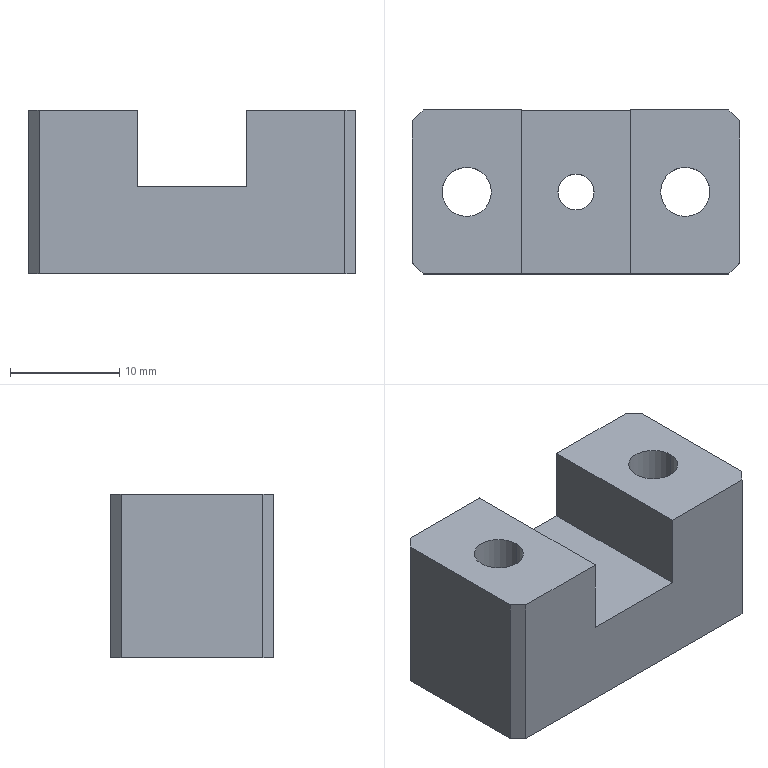Part | STEP file | 03-11 upper blade limit block | 1 solid | 26 faces | box 30 x 15 x 15 mm | volume 4822 mm3 | plane 16 | cylinder 10 | commonest cylinder face diameters 4.5 x4 8 x4 3.3 x2
STEP:
#1=CARTESIAN_POINT('',(-6.,0.,4.4));
#2=VERTEX_POINT('',#1);
#3=CARTESIAN_POINT('',(-14.,0.,4.4));
#4=VERTEX_POINT('',#3);
#5=CARTESIAN_POINT('',(-10.,0.,4.4));
#6=DIRECTION('',(0.,0.,-1.));
#7=DIRECTION('',(-1.,0.,0.));
#8=AXIS2_PLACEMENT_3D('',#5,#6,#7);
#9=CIRCLE('',#8,4.);
#10=EDGE_CURVE('',#2,#4,#9,.T.);
#11=ORIENTED_EDGE('',*,*,#10,.F.);
#12=CARTESIAN_POINT('',(-6.,0.,0.));
#13=VERTEX_POINT('',#12);
#14=CARTESIAN_POINT('',(-6.,0.,0.));
#15=DIRECTION('',(0.,0.,-1.));
#16=VECTOR('',#15,1000.);
#17=LINE('',#14,#16);
#18=EDGE_CURVE('',#2,#13,#17,.T.);
#19=ORIENTED_EDGE('',*,*,#18,.T.);
#20=CARTESIAN_POINT('',(-14.,0.,0.));
#21=VERTEX_POINT('',#20);
#22=CARTESIAN_POINT('',(-10.,0.,0.));
#23=DIRECTION('',(0.,0.,-1.));
#24=DIRECTION('',(-1.,0.,0.));
#25=AXIS2_PLACEMENT_3D('',#22,#23,#24);
#26=CIRCLE('',#25,4.);
#27=EDGE_CURVE('',#13,#21,#26,.T.);
#28=ORIENTED_EDGE('',*,*,#27,.T.);
#29=CARTESIAN_POINT('',(-14.,0.,0.));
#30=DIRECTION('',(0.,0.,-1.));
#31=VECTOR('',#30,1000.);
#32=LINE('',#29,#31);
#33=EDGE_CURVE('',#4,#21,#32,.T.);
#34=ORIENTED_EDGE('',*,*,#33,.F.);
#35=EDGE_LOOP('',(#11,#19,#28,#34));
#36=FACE_OUTER_BOUND('',#35,.T.);
#37=CARTESIAN_POINT('',(-10.,0.,0.));
#38=DIRECTION('',(0.,0.,-1.));
#39=DIRECTION('',(-1.,0.,0.));
#40=AXIS2_PLACEMENT_3D('',#37,#38,#39);
#41=CYLINDRICAL_SURFACE('',#40,4.);
#42=ADVANCED_FACE('',(#36),#41,.F.);
#43=CARTESIAN_POINT('',(-7.75,0.,15.));
#44=VERTEX_POINT('',#43);
#45=CARTESIAN_POINT('',(-12.25,0.,15.));
#46=VERTEX_POINT('',#45);
#47=CARTESIAN_POINT('',(-10.,0.,15.));
#48=DIRECTION('',(0.,0.,-1.));
#49=DIRECTION('',(-1.,0.,0.));
#50=AXIS2_PLACEMENT_3D('',#47,#48,#49);
#51=CIRCLE('',#50,2.25);
#52=EDGE_CURVE('',#44,#46,#51,.T.);
#53=ORIENTED_EDGE('',*,*,#52,.F.);
#54=CARTESIAN_POINT('',(-7.75,0.,4.4));
#55=VERTEX_POINT('',#54);
#56=CARTESIAN_POINT('',(-7.75,0.,0.));
#57=DIRECTION('',(0.,0.,-1.));
#58=VECTOR('',#57,1000.);
#59=LINE('',#56,#58);
#60=EDGE_CURVE('',#44,#55,#59,.T.);
#61=ORIENTED_EDGE('',*,*,#60,.T.);
#62=CARTESIAN_POINT('',(-12.25,0.,4.4));
#63=VERTEX_POINT('',#62);
#64=CARTESIAN_POINT('',(-10.,0.,4.4));
#65=DIRECTION('',(0.,0.,-1.));
#66=DIRECTION('',(-1.,0.,0.));
#67=AXIS2_PLACEMENT_3D('',#64,#65,#66);
#68=CIRCLE('',#67,2.25);
#69=EDGE_CURVE('',#55,#63,#68,.T.);
#70=ORIENTED_EDGE('',*,*,#69,.T.);
#71=CARTESIAN_POINT('',(-12.25,0.,0.));
#72=DIRECTION('',(0.,0.,-1.));
#73=VECTOR('',#72,1000.);
#74=LINE('',#71,#73);
#75=EDGE_CURVE('',#46,#63,#74,.T.);
#76=ORIENTED_EDGE('',*,*,#75,.F.);
#77=EDGE_LOOP('',(#53,#61,#70,#76));
#78=FACE_OUTER_BOUND('',#77,.T.);
#79=CARTESIAN_POINT('',(-10.,0.,0.));
#80=DIRECTION('',(0.,0.,-1.));
#81=DIRECTION('',(-1.,0.,0.));
#82=AXIS2_PLACEMENT_3D('',#79,#80,#81);
#83=CYLINDRICAL_SURFACE('',#82,2.25);
#84=ADVANCED_FACE('',(#78),#83,.F.);
#85=CARTESIAN_POINT('',(14.,0.,4.4));
#86=VERTEX_POINT('',#85);
#87=CARTESIAN_POINT('',(6.,0.,4.4));
#88=VERTEX_POINT('',#87);
#89=CARTESIAN_POINT('',(10.,0.,4.4));
#90=DIRECTION('',(0.,0.,-1.));
#91=DIRECTION('',(-1.,0.,0.));
#92=AXIS2_PLACEMENT_3D('',#89,#90,#91);
#93=CIRCLE('',#92,4.);
#94=EDGE_CURVE('',#86,#88,#93,.T.);
#95=ORIENTED_EDGE('',*,*,#94,.F.);
#96=CARTESIAN_POINT('',(14.,0.,0.));
#97=VERTEX_POINT('',#96);
#98=CARTESIAN_POINT('',(14.,0.,0.));
#99=DIRECTION('',(0.,0.,-1.));
#100=VECTOR('',#99,1000.);
#101=LINE('',#98,#100);
#102=EDGE_CURVE('',#86,#97,#101,.T.);
#103=ORIENTED_EDGE('',*,*,#102,.T.);
#104=CARTESIAN_POINT('',(6.,0.,0.));
#105=VERTEX_POINT('',#104);
#106=CARTESIAN_POINT('',(10.,0.,0.));
#107=DIRECTION('',(0.,0.,-1.));
#108=DIRECTION('',(-1.,0.,0.));
#109=AXIS2_PLACEMENT_3D('',#106,#107,#108);
#110=CIRCLE('',#109,4.);
#111=EDGE_CURVE('',#97,#105,#110,.T.);
#112=ORIENTED_EDGE('',*,*,#111,.T.);
#113=CARTESIAN_POINT('',(6.,0.,0.));
#114=DIRECTION('',(0.,0.,-1.));
#115=VECTOR('',#114,1000.);
#116=LINE('',#113,#115);
#117=EDGE_CURVE('',#88,#105,#116,.T.);
#118=ORIENTED_EDGE('',*,*,#117,.F.);
#119=EDGE_LOOP('',(#95,#103,#112,#118));
#120=FACE_OUTER_BOUND('',#119,.T.);
#121=CARTESIAN_POINT('',(10.,0.,0.));
#122=DIRECTION('',(0.,0.,-1.));
#123=DIRECTION('',(-1.,0.,0.));
#124=AXIS2_PLACEMENT_3D('',#121,#122,#123);
#125=CYLINDRICAL_SURFACE('',#124,4.);
#126=ADVANCED_FACE('',(#120),#125,.F.);
#127=CARTESIAN_POINT('',(12.25,0.,15.));
#128=VERTEX_POINT('',#127);
#129=CARTESIAN_POINT('',(7.75,0.,15.));
#130=VERTEX_POINT('',#129);
#131=CARTESIAN_POINT('',(10.,0.,15.));
#132=DIRECTION('',(0.,0.,-1.));
#133=DIRECTION('',(-1.,0.,0.));
#134=AXIS2_PLACEMENT_3D('',#131,#132,#133);
#135=CIRCLE('',#134,2.25);
#136=EDGE_CURVE('',#128,#130,#135,.T.);
#137=ORIENTED_EDGE('',*,*,#136,.F.);
#138=CARTESIAN_POINT('',(12.25,0.,4.4));
#139=VERTEX_POINT('',#138);
#140=CARTESIAN_POINT('',(12.25,0.,0.));
#141=DIRECTION('',(0.,0.,-1.));
#142=VECTOR('',#141,1000.);
#143=LINE('',#140,#142);
#144=EDGE_CURVE('',#128,#139,#143,.T.);
#145=ORIENTED_EDGE('',*,*,#144,.T.);
#146=CARTESIAN_POINT('',(7.75,0.,4.4));
#147=VERTEX_POINT('',#146);
#148=CARTESIAN_POINT('',(10.,0.,4.4));
#149=DIRECTION('',(0.,0.,-1.));
#150=DIRECTION('',(-1.,0.,0.));
#151=AXIS2_PLACEMENT_3D('',#148,#149,#150);
#152=CIRCLE('',#151,2.25);
#153=EDGE_CURVE('',#139,#147,#152,.T.);
#154=ORIENTED_EDGE('',*,*,#153,.T.);
#155=CARTESIAN_POINT('',(7.75,0.,0.));
#156=DIRECTION('',(0.,0.,-1.));
#157=VECTOR('',#156,1000.);
#158=LINE('',#155,#157);
#159=EDGE_CURVE('',#130,#147,#158,.T.);
#160=ORIENTED_EDGE('',*,*,#159,.F.);
#161=EDGE_LOOP('',(#137,#145,#154,#160));
#162=FACE_OUTER_BOUND('',#161,.T.);
#163=CARTESIAN_POINT('',(10.,0.,0.));
#164=DIRECTION('',(0.,0.,-1.));
#165=DIRECTION('',(-1.,0.,0.));
#166=AXIS2_PLACEMENT_3D('',#163,#164,#165);
#167=CYLINDRICAL_SURFACE('',#166,2.25);
#168=ADVANCED_FACE('',(#162),#167,.F.);
#169=CARTESIAN_POINT('',(1.65,0.,8.));
#170=VERTEX_POINT('',#169);
#171=CARTESIAN_POINT('',(-1.65,0.,8.));
#172=VERTEX_POINT('',#171);
#173=CARTESIAN_POINT('',(0.,0.,8.));
#174=DIRECTION('',(0.,0.,-1.));
#175=DIRECTION('',(-1.,0.,0.));
#176=AXIS2_PLACEMENT_3D('',#173,#174,#175);
#177=CIRCLE('',#176,1.65);
#178=EDGE_CURVE('',#170,#172,#177,.T.);
#179=ORIENTED_EDGE('',*,*,#178,.F.);
#180=CARTESIAN_POINT('',(1.65,0.,0.));
#181=VERTEX_POINT('',#180);
#182=CARTESIAN_POINT('',(1.65,0.,0.));
#183=DIRECTION('',(0.,0.,-1.));
#184=VECTOR('',#183,1000.);
#185=LINE('',#182,#184);
#186=EDGE_CURVE('',#170,#181,#185,.T.);
#187=ORIENTED_EDGE('',*,*,#186,.T.);
#188=CARTESIAN_POINT('',(-1.65,0.,0.));
#189=VERTEX_POINT('',#188);
#190=CARTESIAN_POINT('',(0.,0.,0.));
#191=DIRECTION('',(0.,0.,-1.));
#192=DIRECTION('',(-1.,0.,0.));
#193=AXIS2_PLACEMENT_3D('',#190,#191,#192);
#194=CIRCLE('',#193,1.65);
#195=EDGE_CURVE('',#181,#189,#194,.T.);
#196=ORIENTED_EDGE('',*,*,#195,.T.);
#197=CARTESIAN_POINT('',(-1.65,0.,0.));
#198=DIRECTION('',(0.,0.,-1.));
#199=VECTOR('',#198,1000.);
#200=LINE('',#197,#199);
#201=EDGE_CURVE('',#172,#189,#200,.T.);
#202=ORIENTED_EDGE('',*,*,#201,.F.);
#203=EDGE_LOOP('',(#179,#187,#196,#202));
#204=FACE_OUTER_BOUND('',#203,.T.);
#205=CARTESIAN_POINT('',(0.,0.,0.));
#206=DIRECTION('',(0.,0.,-1.));
#207=DIRECTION('',(-1.,0.,0.));
#208=AXIS2_PLACEMENT_3D('',#205,#206,#207);
#209=CYLINDRICAL_SURFACE('',#208,1.65);
#210=ADVANCED_FACE('',(#204),#209,.F.);
#211=CARTESIAN_POINT('',(-10.,0.,15.));
#212=DIRECTION('',(0.,0.,-1.));
#213=DIRECTION('',(-1.,0.,0.));
#214=AXIS2_PLACEMENT_3D('',#211,#212,#213);
#215=CIRCLE('',#214,2.25);
#216=EDGE_CURVE('',#46,#44,#215,.T.);
#217=ORIENTED_EDGE('',*,*,#216,.T.);
#218=ORIENTED_EDGE('',*,*,#52,.T.);
#219=EDGE_LOOP('',(#217,#218));
#220=FACE_BOUND('',#219,.T.);
#221=CARTESIAN_POINT('',(-15.,6.5,15.));
#222=VERTEX_POINT('',#221);
#223=CARTESIAN_POINT('',(-15.,-6.5,15.));
#224=VERTEX_POINT('',#223);
#225=CARTESIAN_POINT('',(-15.,7.5,15.));
#226=DIRECTION('',(0.,-1.,0.));
#227=VECTOR('',#226,1000.);
#228=LINE('',#225,#227);
#229=EDGE_CURVE('',#222,#224,#228,.T.);
#230=ORIENTED_EDGE('',*,*,#229,.T.);
#231=CARTESIAN_POINT('',(-14.,-7.5,15.));
#232=VERTEX_POINT('',#231);
#233=CARTESIAN_POINT('',(0.5,-22.,15.));
#234=DIRECTION('',(0.7071,-0.7071,0.));
#235=VECTOR('',#234,1000.);
#236=LINE('',#233,#235);
#237=EDGE_CURVE('',#224,#232,#236,.T.);
#238=ORIENTED_EDGE('',*,*,#237,.T.);
#239=CARTESIAN_POINT('',(-5.,-7.5,15.));
#240=VERTEX_POINT('',#239);
#241=CARTESIAN_POINT('',(-15.,-7.5,15.));
#242=DIRECTION('',(1.,0.,0.));
#243=VECTOR('',#242,1000.);
#244=LINE('',#241,#243);
#245=EDGE_CURVE('',#232,#240,#244,.T.);
#246=ORIENTED_EDGE('',*,*,#245,.T.);
#247=CARTESIAN_POINT('',(-5.,7.5,15.));
#248=VERTEX_POINT('',#247);
#249=CARTESIAN_POINT('',(-5.,7.5,15.));
#250=DIRECTION('',(0.,-1.,0.));
#251=VECTOR('',#250,1000.);
#252=LINE('',#249,#251);
#253=EDGE_CURVE('',#248,#240,#252,.T.);
#254=ORIENTED_EDGE('',*,*,#253,.F.);
#255=CARTESIAN_POINT('',(-14.,7.5,15.));
#256=VERTEX_POINT('',#255);
#257=CARTESIAN_POINT('',(-15.,7.5,15.));
#258=DIRECTION('',(-1.,0.,0.));
#259=VECTOR('',#258,1000.);
#260=LINE('',#257,#259);
#261=EDGE_CURVE('',#248,#256,#260,.T.);
#262=ORIENTED_EDGE('',*,*,#261,.T.);
#263=CARTESIAN_POINT('',(-7.,14.5,15.));
#264=DIRECTION('',(-0.7071,-0.7071,0.));
#265=VECTOR('',#264,1000.);
#266=LINE('',#263,#265);
#267=EDGE_CURVE('',#256,#222,#266,.T.);
#268=ORIENTED_EDGE('',*,*,#267,.T.);
#269=EDGE_LOOP('',(#230,#238,#246,#254,#262,#268));
#270=FACE_OUTER_BOUND('',#269,.T.);
#271=CARTESIAN_POINT('',(15.,-7.5,15.));
#272=DIRECTION('',(0.,0.,1.));
#273=DIRECTION('',(1.,0.,0.));
#274=AXIS2_PLACEMENT_3D('',#271,#272,#273);
#275=PLANE('',#274);
#276=ADVANCED_FACE('',(#220,#270),#275,.T.);
#277=CARTESIAN_POINT('',(15.,-6.5,15.));
#278=VERTEX_POINT('',#277);
#279=CARTESIAN_POINT('',(15.,6.5,15.));
#280=VERTEX_POINT('',#279);
#281=CARTESIAN_POINT('',(15.,7.5,15.));
#282=DIRECTION('',(0.,1.,0.));
#283=VECTOR('',#282,1000.);
#284=LINE('',#281,#283);
#285=EDGE_CURVE('',#278,#280,#284,.T.);
#286=ORIENTED_EDGE('',*,*,#285,.F.);
#287=CARTESIAN_POINT('',(15.,-6.5,0.));
#288=VERTEX_POINT('',#287);
#289=CARTESIAN_POINT('',(15.,-6.5,15.));
#290=DIRECTION('',(0.,0.,-1.));
#291=VECTOR('',#290,1000.);
#292=LINE('',#289,#291);
#293=EDGE_CURVE('',#278,#288,#292,.T.);
#294=ORIENTED_EDGE('',*,*,#293,.T.);
#295=CARTESIAN_POINT('',(15.,6.5,0.));
#296=VERTEX_POINT('',#295);
#297=CARTESIAN_POINT('',(15.,7.5,0.));
#298=DIRECTION('',(0.,1.,0.));
#299=VECTOR('',#298,1000.);
#300=LINE('',#297,#299);
#301=EDGE_CURVE('',#288,#296,#300,.T.);
#302=ORIENTED_EDGE('',*,*,#301,.T.);
#303=CARTESIAN_POINT('',(15.,6.5,15.));
#304=DIRECTION('',(0.,0.,1.));
#305=VECTOR('',#304,1000.);
#306=LINE('',#303,#305);
#307=EDGE_CURVE('',#296,#280,#306,.T.);
#308=ORIENTED_EDGE('',*,*,#307,.T.);
#309=EDGE_LOOP('',(#286,#294,#302,#308));
#310=FACE_OUTER_BOUND('',#309,.T.);
#311=CARTESIAN_POINT('',(15.,7.5,15.));
#312=DIRECTION('',(-1.,0.,0.));
#313=DIRECTION('',(0.,-1.,0.));
#314=AXIS2_PLACEMENT_3D('',#311,#312,#313);
#315=PLANE('',#314);
#316=ADVANCED_FACE('',(#310),#315,.F.);
#317=CARTESIAN_POINT('',(14.,7.5,15.));
#318=VERTEX_POINT('',#317);
#319=CARTESIAN_POINT('',(5.,7.5,15.));
#320=VERTEX_POINT('',#319);
#321=CARTESIAN_POINT('',(-15.,7.5,15.));
#322=DIRECTION('',(-1.,0.,0.));
#323=VECTOR('',#322,1000.);
#324=LINE('',#321,#323);
#325=EDGE_CURVE('',#318,#320,#324,.T.);
#326=ORIENTED_EDGE('',*,*,#325,.F.);
#327=CARTESIAN_POINT('',(14.,7.5,0.));
#328=VERTEX_POINT('',#327);
#329=CARTESIAN_POINT('',(14.,7.5,15.));
#330=DIRECTION('',(0.,0.,-1.));
#331=VECTOR('',#330,1000.);
#332=LINE('',#329,#331);
#333=EDGE_CURVE('',#318,#328,#332,.T.);
#334=ORIENTED_EDGE('',*,*,#333,.T.);
#335=CARTESIAN_POINT('',(-14.,7.5,0.));
#336=VERTEX_POINT('',#335);
#337=CARTESIAN_POINT('',(-15.,7.5,0.));
#338=DIRECTION('',(-1.,0.,0.));
#339=VECTOR('',#338,1000.);
#340=LINE('',#337,#339);
#341=EDGE_CURVE('',#328,#336,#340,.T.);
#342=ORIENTED_EDGE('',*,*,#341,.T.);
#343=CARTESIAN_POINT('',(-14.,7.5,15.));
#344=DIRECTION('',(0.,0.,1.));
#345=VECTOR('',#344,1000.);
#346=LINE('',#343,#345);
#347=EDGE_CURVE('',#336,#256,#346,.T.);
#348=ORIENTED_EDGE('',*,*,#347,.T.);
#349=ORIENTED_EDGE('',*,*,#261,.F.);
#350=CARTESIAN_POINT('',(-5.,7.5,8.));
#351=VERTEX_POINT('',#350);
#352=CARTESIAN_POINT('',(-5.,7.5,15.));
#353=DIRECTION('',(0.,0.,-1.));
#354=VECTOR('',#353,1000.);
#355=LINE('',#352,#354);
#356=EDGE_CURVE('',#248,#351,#355,.T.);
#357=ORIENTED_EDGE('',*,*,#356,.T.);
#358=CARTESIAN_POINT('',(5.,7.5,8.));
#359=VERTEX_POINT('',#358);
#360=CARTESIAN_POINT('',(-5.,7.5,8.));
#361=DIRECTION('',(1.,0.,0.));
#362=VECTOR('',#361,1000.);
#363=LINE('',#360,#362);
#364=EDGE_CURVE('',#351,#359,#363,.T.);
#365=ORIENTED_EDGE('',*,*,#364,.T.);
#366=CARTESIAN_POINT('',(5.,7.5,15.));
#367=DIRECTION('',(0.,0.,1.));
#368=VECTOR('',#367,1000.);
#369=LINE('',#366,#368);
#370=EDGE_CURVE('',#359,#320,#369,.T.);
#371=ORIENTED_EDGE('',*,*,#370,.T.);
#372=EDGE_LOOP('',(#326,#334,#342,#348,#349,#357,#365,#371));
#373=FACE_OUTER_BOUND('',#372,.T.);
#374=CARTESIAN_POINT('',(-15.,7.5,15.));
#375=DIRECTION('',(0.,-1.,0.));
#376=DIRECTION('',(0.,0.,-1.));
#377=AXIS2_PLACEMENT_3D('',#374,#375,#376);
#378=PLANE('',#377);
#379=ADVANCED_FACE('',(#373),#378,.F.);
#380=CARTESIAN_POINT('',(-15.,6.5,0.));
#381=VERTEX_POINT('',#380);
#382=CARTESIAN_POINT('',(-15.,-6.5,0.));
#383=VERTEX_POINT('',#382);
#384=CARTESIAN_POINT('',(-15.,7.5,0.));
#385=DIRECTION('',(0.,-1.,0.));
#386=VECTOR('',#385,1000.);
#387=LINE('',#384,#386);
#388=EDGE_CURVE('',#381,#383,#387,.T.);
#389=ORIENTED_EDGE('',*,*,#388,.T.);
#390=CARTESIAN_POINT('',(-15.,-6.5,15.));
#391=DIRECTION('',(0.,0.,1.));
#392=VECTOR('',#391,1000.);
#393=LINE('',#390,#392);
#394=EDGE_CURVE('',#383,#224,#393,.T.);
#395=ORIENTED_EDGE('',*,*,#394,.T.);
#396=ORIENTED_EDGE('',*,*,#229,.F.);
#397=CARTESIAN_POINT('',(-15.,6.5,15.));
#398=DIRECTION('',(0.,0.,-1.));
#399=VECTOR('',#398,1000.);
#400=LINE('',#397,#399);
#401=EDGE_CURVE('',#222,#381,#400,.T.);
#402=ORIENTED_EDGE('',*,*,#401,.T.);
#403=EDGE_LOOP('',(#389,#395,#396,#402));
#404=FACE_OUTER_BOUND('',#403,.T.);
#405=CARTESIAN_POINT('',(-15.,7.5,15.));
#406=DIRECTION('',(1.,0.,0.));
#407=DIRECTION('',(0.,1.,0.));
#408=AXIS2_PLACEMENT_3D('',#405,#406,#407);
#409=PLANE('',#408);
#410=ADVANCED_FACE('',(#404),#409,.F.);
#411=ORIENTED_EDGE('',*,*,#245,.F.);
#412=CARTESIAN_POINT('',(-14.,-7.5,0.));
#413=VERTEX_POINT('',#412);
#414=CARTESIAN_POINT('',(-14.,-7.5,15.));
#415=DIRECTION('',(0.,0.,-1.));
#416=VECTOR('',#415,1000.);
#417=LINE('',#414,#416);
#418=EDGE_CURVE('',#232,#413,#417,.T.);
#419=ORIENTED_EDGE('',*,*,#418,.T.);
#420=CARTESIAN_POINT('',(14.,-7.5,0.));
#421=VERTEX_POINT('',#420);
#422=CARTESIAN_POINT('',(-15.,-7.5,0.));
#423=DIRECTION('',(1.,0.,0.));
#424=VECTOR('',#423,1000.);
#425=LINE('',#422,#424);
#426=EDGE_CURVE('',#413,#421,#425,.T.);
#427=ORIENTED_EDGE('',*,*,#426,.T.);
#428=CARTESIAN_POINT('',(14.,-7.5,15.));
#429=VERTEX_POINT('',#428);
#430=CARTESIAN_POINT('',(14.,-7.5,15.));
#431=DIRECTION('',(0.,0.,1.));
#432=VECTOR('',#431,1000.);
#433=LINE('',#430,#432);
#434=EDGE_CURVE('',#421,#429,#433,.T.);
#435=ORIENTED_EDGE('',*,*,#434,.T.);
#436=CARTESIAN_POINT('',(5.,-7.5,15.));
#437=VERTEX_POINT('',#436);
#438=CARTESIAN_POINT('',(-15.,-7.5,15.));
#439=DIRECTION('',(1.,0.,0.));
#440=VECTOR('',#439,1000.);
#441=LINE('',#438,#440);
#442=EDGE_CURVE('',#437,#429,#441,.T.);
#443=ORIENTED_EDGE('',*,*,#442,.F.);
#444=CARTESIAN_POINT('',(5.,-7.5,8.));
#445=VERTEX_POINT('',#444);
#446=CARTESIAN_POINT('',(5.,-7.5,15.));
#447=DIRECTION('',(0.,0.,1.));
#448=VECTOR('',#447,1000.);
#449=LINE('',#446,#448);
#450=EDGE_CURVE('',#445,#437,#449,.T.);
#451=ORIENTED_EDGE('',*,*,#450,.F.);
#452=CARTESIAN_POINT('',(-5.,-7.5,8.));
#453=VERTEX_POINT('',#452);
#454=CARTESIAN_POINT('',(-5.,-7.5,8.));
#455=DIRECTION('',(1.,0.,0.));
#456=VECTOR('',#455,1000.);
#457=LINE('',#454,#456);
#458=EDGE_CURVE('',#453,#445,#457,.T.);
#459=ORIENTED_EDGE('',*,*,#458,.F.);
#460=CARTESIAN_POINT('',(-5.,-7.5,15.));
#461=DIRECTION('',(0.,0.,-1.));
#462=VECTOR('',#461,1000.);
#463=LINE('',#460,#462);
#464=EDGE_CURVE('',#240,#453,#463,.T.);
#465=ORIENTED_EDGE('',*,*,#464,.F.);
#466=EDGE_LOOP('',(#411,#419,#427,#435,#443,#451,#459,#465));
#467=FACE_OUTER_BOUND('',#466,.T.);
#468=CARTESIAN_POINT('',(-15.,-7.5,15.));
#469=DIRECTION('',(0.,1.,0.));
#470=DIRECTION('',(0.,0.,1.));
#471=AXIS2_PLACEMENT_3D('',#468,#469,#470);
#472=PLANE('',#471);
#473=ADVANCED_FACE('',(#467),#472,.F.);
#474=CARTESIAN_POINT('',(10.,0.,15.));
#475=DIRECTION('',(0.,0.,-1.));
#476=DIRECTION('',(-1.,0.,0.));
#477=AXIS2_PLACEMENT_3D('',#474,#475,#476);
#478=CIRCLE('',#477,2.25);
#479=EDGE_CURVE('',#130,#128,#478,.T.);
#480=ORIENTED_EDGE('',*,*,#479,.T.);
#481=ORIENTED_EDGE('',*,*,#136,.T.);
#482=EDGE_LOOP('',(#480,#481));
#483=FACE_BOUND('',#482,.T.);
#484=ORIENTED_EDGE('',*,*,#442,.T.);
#485=CARTESIAN_POINT('',(14.5,-7.,15.));
#486=DIRECTION('',(0.7071,0.7071,0.));
#487=VECTOR('',#486,1000.);
#488=LINE('',#485,#487);
#489=EDGE_CURVE('',#429,#278,#488,.T.);
#490=ORIENTED_EDGE('',*,*,#489,.T.);
#491=ORIENTED_EDGE('',*,*,#285,.T.);
#492=CARTESIAN_POINT('',(22.,-0.5,15.));
#493=DIRECTION('',(-0.7071,0.7071,0.));
#494=VECTOR('',#493,1000.);
#495=LINE('',#492,#494);
#496=EDGE_CURVE('',#280,#318,#495,.T.);
#497=ORIENTED_EDGE('',*,*,#496,.T.);
#498=ORIENTED_EDGE('',*,*,#325,.T.);
#499=CARTESIAN_POINT('',(5.,7.5,15.));
#500=DIRECTION('',(0.,-1.,0.));
#501=VECTOR('',#500,1000.);
#502=LINE('',#499,#501);
#503=EDGE_CURVE('',#320,#437,#502,.T.);
#504=ORIENTED_EDGE('',*,*,#503,.T.);
#505=EDGE_LOOP('',(#484,#490,#491,#497,#498,#504));
#506=FACE_OUTER_BOUND('',#505,.T.);
#507=CARTESIAN_POINT('',(15.,-7.5,15.));
#508=DIRECTION('',(0.,0.,1.));
#509=DIRECTION('',(1.,0.,0.));
#510=AXIS2_PLACEMENT_3D('',#507,#508,#509);
#511=PLANE('',#510);
#512=ADVANCED_FACE('',(#483,#506),#511,.T.);
#513=CARTESIAN_POINT('',(-10.,0.,0.));
#514=DIRECTION('',(0.,0.,-1.));
#515=DIRECTION('',(-1.,0.,0.));
#516=AXIS2_PLACEMENT_3D('',#513,#514,#515);
#517=CIRCLE('',#516,4.);
#518=EDGE_CURVE('',#21,#13,#517,.T.);
#519=ORIENTED_EDGE('',*,*,#518,.F.);
#520=ORIENTED_EDGE('',*,*,#27,.F.);
#521=EDGE_LOOP('',(#519,#520));
#522=FACE_BOUND('',#521,.T.);
#523=CARTESIAN_POINT('',(10.,0.,0.));
#524=DIRECTION('',(0.,0.,-1.));
#525=DIRECTION('',(-1.,0.,0.));
#526=AXIS2_PLACEMENT_3D('',#523,#524,#525);
#527=CIRCLE('',#526,4.);
#528=EDGE_CURVE('',#105,#97,#527,.T.);
#529=ORIENTED_EDGE('',*,*,#528,.F.);
#530=ORIENTED_EDGE('',*,*,#111,.F.);
#531=EDGE_LOOP('',(#529,#530));
#532=FACE_BOUND('',#531,.T.);
#533=CARTESIAN_POINT('',(0.,0.,0.));
#534=DIRECTION('',(0.,0.,-1.));
#535=DIRECTION('',(-1.,0.,0.));
#536=AXIS2_PLACEMENT_3D('',#533,#534,#535);
#537=CIRCLE('',#536,1.65);
#538=EDGE_CURVE('',#189,#181,#537,.T.);
#539=ORIENTED_EDGE('',*,*,#538,.F.);
#540=ORIENTED_EDGE('',*,*,#195,.F.);
#541=EDGE_LOOP('',(#539,#540));
#542=FACE_BOUND('',#541,.T.);
#543=ORIENTED_EDGE('',*,*,#426,.F.);
#544=CARTESIAN_POINT('',(-14.,-7.5,0.));
#545=DIRECTION('',(-0.7071,0.7071,0.));
#546=VECTOR('',#545,1000.);
#547=LINE('',#544,#546);
#548=EDGE_CURVE('',#413,#383,#547,.T.);
#549=ORIENTED_EDGE('',*,*,#548,.T.);
#550=ORIENTED_EDGE('',*,*,#388,.F.);
#551=CARTESIAN_POINT('',(-15.,6.5,0.));
#552=DIRECTION('',(0.7071,0.7071,0.));
#553=VECTOR('',#552,1000.);
#554=LINE('',#551,#553);
#555=EDGE_CURVE('',#381,#336,#554,.T.);
#556=ORIENTED_EDGE('',*,*,#555,.T.);
#557=ORIENTED_EDGE('',*,*,#341,.F.);
#558=CARTESIAN_POINT('',(14.,7.5,0.));
#559=DIRECTION('',(0.7071,-0.7071,0.));
#560=VECTOR('',#559,1000.);
#561=LINE('',#558,#560);
#562=EDGE_CURVE('',#328,#296,#561,.T.);
#563=ORIENTED_EDGE('',*,*,#562,.T.);
#564=ORIENTED_EDGE('',*,*,#301,.F.);
#565=CARTESIAN_POINT('',(15.,-6.5,0.));
#566=DIRECTION('',(-0.7071,-0.7071,0.));
#567=VECTOR('',#566,1000.);
#568=LINE('',#565,#567);
#569=EDGE_CURVE('',#288,#421,#568,.T.);
#570=ORIENTED_EDGE('',*,*,#569,.T.);
#571=EDGE_LOOP('',(#543,#549,#550,#556,#557,#563,#564,#570));
#572=FACE_OUTER_BOUND('',#571,.T.);
#573=CARTESIAN_POINT('',(15.,-7.5,0.));
#574=DIRECTION('',(0.,0.,1.));
#575=DIRECTION('',(1.,0.,0.));
#576=AXIS2_PLACEMENT_3D('',#573,#574,#575);
#577=PLANE('',#576);
#578=ADVANCED_FACE('',(#522,#532,#542,#572),#577,.F.);
#579=ORIENTED_EDGE('',*,*,#464,.T.);
#580=CARTESIAN_POINT('',(-5.,7.5,8.));
#581=DIRECTION('',(0.,-1.,0.));
#582=VECTOR('',#581,1000.);
#583=LINE('',#580,#582);
#584=EDGE_CURVE('',#351,#453,#583,.T.);
#585=ORIENTED_EDGE('',*,*,#584,.F.);
#586=ORIENTED_EDGE('',*,*,#356,.F.);
#587=ORIENTED_EDGE('',*,*,#253,.T.);
#588=EDGE_LOOP('',(#579,#585,#586,#587));
#589=FACE_OUTER_BOUND('',#588,.T.);
#590=CARTESIAN_POINT('',(-5.,7.5,15.));
#591=DIRECTION('',(-1.,0.,0.));
#592=DIRECTION('',(0.,0.,1.));
#593=AXIS2_PLACEMENT_3D('',#590,#591,#592);
#594=PLANE('',#593);
#595=ADVANCED_FACE('',(#589),#594,.F.);
#596=ORIENTED_EDGE('',*,*,#450,.T.);
#597=ORIENTED_EDGE('',*,*,#503,.F.);
#598=ORIENTED_EDGE('',*,*,#370,.F.);
#599=CARTESIAN_POINT('',(5.,7.5,8.));
#600=DIRECTION('',(0.,-1.,0.));
#601=VECTOR('',#600,1000.);
#602=LINE('',#599,#601);
#603=EDGE_CURVE('',#359,#445,#602,.T.);
#604=ORIENTED_EDGE('',*,*,#603,.T.);
#605=EDGE_LOOP('',(#596,#597,#598,#604));
#606=FACE_OUTER_BOUND('',#605,.T.);
#607=CARTESIAN_POINT('',(5.,7.5,15.));
#608=DIRECTION('',(1.,0.,0.));
#609=DIRECTION('',(0.,0.,-1.));
#610=AXIS2_PLACEMENT_3D('',#607,#608,#609);
#611=PLANE('',#610);
#612=ADVANCED_FACE('',(#606),#611,.F.);
#613=CARTESIAN_POINT('',(0.,0.,8.));
#614=DIRECTION('',(0.,0.,-1.));
#615=DIRECTION('',(-1.,0.,0.));
#616=AXIS2_PLACEMENT_3D('',#613,#614,#615);
#617=CIRCLE('',#616,1.65);
#618=EDGE_CURVE('',#172,#170,#617,.T.);
#619=ORIENTED_EDGE('',*,*,#618,.T.);
#620=ORIENTED_EDGE('',*,*,#178,.T.);
#621=EDGE_LOOP('',(#619,#620));
#622=FACE_BOUND('',#621,.T.);
#623=ORIENTED_EDGE('',*,*,#458,.T.);
#624=ORIENTED_EDGE('',*,*,#603,.F.);
#625=ORIENTED_EDGE('',*,*,#364,.F.);
#626=ORIENTED_EDGE('',*,*,#584,.T.);
#627=EDGE_LOOP('',(#623,#624,#625,#626));
#628=FACE_OUTER_BOUND('',#627,.T.);
#629=CARTESIAN_POINT('',(-5.,7.5,8.));
#630=DIRECTION('',(0.,0.,-1.));
#631=DIRECTION('',(-1.,0.,0.));
#632=AXIS2_PLACEMENT_3D('',#629,#630,#631);
#633=PLANE('',#632);
#634=ADVANCED_FACE('',(#622,#628),#633,.F.);
#635=ORIENTED_EDGE('',*,*,#186,.F.);
#636=ORIENTED_EDGE('',*,*,#618,.F.);
#637=ORIENTED_EDGE('',*,*,#201,.T.);
#638=ORIENTED_EDGE('',*,*,#538,.T.);
#639=EDGE_LOOP('',(#635,#636,#637,#638));
#640=FACE_OUTER_BOUND('',#639,.T.);
#641=CARTESIAN_POINT('',(0.,0.,0.));
#642=DIRECTION('',(0.,0.,-1.));
#643=DIRECTION('',(-1.,0.,0.));
#644=AXIS2_PLACEMENT_3D('',#641,#642,#643);
#645=CYLINDRICAL_SURFACE('',#644,1.65);
#646=ADVANCED_FACE('',(#640),#645,.F.);
#647=ORIENTED_EDGE('',*,*,#237,.F.);
#648=ORIENTED_EDGE('',*,*,#394,.F.);
#649=ORIENTED_EDGE('',*,*,#548,.F.);
#650=ORIENTED_EDGE('',*,*,#418,.F.);
#651=EDGE_LOOP('',(#647,#648,#649,#650));
#652=FACE_OUTER_BOUND('',#651,.T.);
#653=CARTESIAN_POINT('',(-14.,-7.5,15.));
#654=DIRECTION('',(0.7071,0.7071,0.));
#655=DIRECTION('',(-0.7071,0.7071,0.));
#656=AXIS2_PLACEMENT_3D('',#653,#654,#655);
#657=PLANE('',#656);
#658=ADVANCED_FACE('',(#652),#657,.F.);
#659=ORIENTED_EDGE('',*,*,#489,.F.);
#660=ORIENTED_EDGE('',*,*,#434,.F.);
#661=ORIENTED_EDGE('',*,*,#569,.F.);
#662=ORIENTED_EDGE('',*,*,#293,.F.);
#663=EDGE_LOOP('',(#659,#660,#661,#662));
#664=FACE_OUTER_BOUND('',#663,.T.);
#665=CARTESIAN_POINT('',(15.,-6.5,15.));
#666=DIRECTION('',(-0.7071,0.7071,0.));
#667=DIRECTION('',(-0.7071,-0.7071,0.));
#668=AXIS2_PLACEMENT_3D('',#665,#666,#667);
#669=PLANE('',#668);
#670=ADVANCED_FACE('',(#664),#669,.F.);
#671=ORIENTED_EDGE('',*,*,#496,.F.);
#672=ORIENTED_EDGE('',*,*,#307,.F.);
#673=ORIENTED_EDGE('',*,*,#562,.F.);
#674=ORIENTED_EDGE('',*,*,#333,.F.);
#675=EDGE_LOOP('',(#671,#672,#673,#674));
#676=FACE_OUTER_BOUND('',#675,.T.);
#677=CARTESIAN_POINT('',(14.,7.5,15.));
#678=DIRECTION('',(-0.7071,-0.7071,0.));
#679=DIRECTION('',(0.7071,-0.7071,0.));
#680=AXIS2_PLACEMENT_3D('',#677,#678,#679);
#681=PLANE('',#680);
#682=ADVANCED_FACE('',(#676),#681,.F.);
#683=ORIENTED_EDGE('',*,*,#267,.F.);
#684=ORIENTED_EDGE('',*,*,#347,.F.);
#685=ORIENTED_EDGE('',*,*,#555,.F.);
#686=ORIENTED_EDGE('',*,*,#401,.F.);
#687=EDGE_LOOP('',(#683,#684,#685,#686));
#688=FACE_OUTER_BOUND('',#687,.T.);
#689=CARTESIAN_POINT('',(-15.,6.5,15.));
#690=DIRECTION('',(0.7071,-0.7071,0.));
#691=DIRECTION('',(0.7071,0.7071,0.));
#692=AXIS2_PLACEMENT_3D('',#689,#690,#691);
#693=PLANE('',#692);
#694=ADVANCED_FACE('',(#688),#693,.F.);
#695=ORIENTED_EDGE('',*,*,#144,.F.);
#696=ORIENTED_EDGE('',*,*,#479,.F.);
#697=ORIENTED_EDGE('',*,*,#159,.T.);
#698=CARTESIAN_POINT('',(10.,0.,4.4));
#699=DIRECTION('',(0.,0.,-1.));
#700=DIRECTION('',(-1.,0.,0.));
#701=AXIS2_PLACEMENT_3D('',#698,#699,#700);
#702=CIRCLE('',#701,2.25);
#703=EDGE_CURVE('',#147,#139,#702,.T.);
#704=ORIENTED_EDGE('',*,*,#703,.T.);
#705=EDGE_LOOP('',(#695,#696,#697,#704));
#706=FACE_OUTER_BOUND('',#705,.T.);
#707=CARTESIAN_POINT('',(10.,0.,0.));
#708=DIRECTION('',(0.,0.,-1.));
#709=DIRECTION('',(-1.,0.,0.));
#710=AXIS2_PLACEMENT_3D('',#707,#708,#709);
#711=CYLINDRICAL_SURFACE('',#710,2.25);
#712=ADVANCED_FACE('',(#706),#711,.F.);
#713=ORIENTED_EDGE('',*,*,#703,.F.);
#714=ORIENTED_EDGE('',*,*,#153,.F.);
#715=EDGE_LOOP('',(#713,#714));
#716=FACE_BOUND('',#715,.T.);
#717=CARTESIAN_POINT('',(10.,0.,4.4));
#718=DIRECTION('',(0.,0.,-1.));
#719=DIRECTION('',(-1.,0.,0.));
#720=AXIS2_PLACEMENT_3D('',#717,#718,#719);
#721=CIRCLE('',#720,4.);
#722=EDGE_CURVE('',#88,#86,#721,.T.);
#723=ORIENTED_EDGE('',*,*,#722,.T.);
#724=ORIENTED_EDGE('',*,*,#94,.T.);
#725=EDGE_LOOP('',(#723,#724));
#726=FACE_OUTER_BOUND('',#725,.T.);
#727=CARTESIAN_POINT('',(12.25,0.,4.4));
#728=DIRECTION('',(0.,0.,1.));
#729=DIRECTION('',(1.,0.,0.));
#730=AXIS2_PLACEMENT_3D('',#727,#728,#729);
#731=PLANE('',#730);
#732=ADVANCED_FACE('',(#716,#726),#731,.F.);
#733=ORIENTED_EDGE('',*,*,#102,.F.);
#734=ORIENTED_EDGE('',*,*,#722,.F.);
#735=ORIENTED_EDGE('',*,*,#117,.T.);
#736=ORIENTED_EDGE('',*,*,#528,.T.);
#737=EDGE_LOOP('',(#733,#734,#735,#736));
#738=FACE_OUTER_BOUND('',#737,.T.);
#739=CARTESIAN_POINT('',(10.,0.,0.));
#740=DIRECTION('',(0.,0.,-1.));
#741=DIRECTION('',(-1.,0.,0.));
#742=AXIS2_PLACEMENT_3D('',#739,#740,#741);
#743=CYLINDRICAL_SURFACE('',#742,4.);
#744=ADVANCED_FACE('',(#738),#743,.F.);
#745=ORIENTED_EDGE('',*,*,#60,.F.);
#746=ORIENTED_EDGE('',*,*,#216,.F.);
#747=ORIENTED_EDGE('',*,*,#75,.T.);
#748=CARTESIAN_POINT('',(-10.,0.,4.4));
#749=DIRECTION('',(0.,0.,-1.));
#750=DIRECTION('',(-1.,0.,0.));
#751=AXIS2_PLACEMENT_3D('',#748,#749,#750);
#752=CIRCLE('',#751,2.25);
#753=EDGE_CURVE('',#63,#55,#752,.T.);
#754=ORIENTED_EDGE('',*,*,#753,.T.);
#755=EDGE_LOOP('',(#745,#746,#747,#754));
#756=FACE_OUTER_BOUND('',#755,.T.);
#757=CARTESIAN_POINT('',(-10.,0.,0.));
#758=DIRECTION('',(0.,0.,-1.));
#759=DIRECTION('',(-1.,0.,0.));
#760=AXIS2_PLACEMENT_3D('',#757,#758,#759);
#761=CYLINDRICAL_SURFACE('',#760,2.25);
#762=ADVANCED_FACE('',(#756),#761,.F.);
#763=ORIENTED_EDGE('',*,*,#753,.F.);
#764=ORIENTED_EDGE('',*,*,#69,.F.);
#765=EDGE_LOOP('',(#763,#764));
#766=FACE_BOUND('',#765,.T.);
#767=CARTESIAN_POINT('',(-10.,0.,4.4));
#768=DIRECTION('',(0.,0.,-1.));
#769=DIRECTION('',(-1.,0.,0.));
#770=AXIS2_PLACEMENT_3D('',#767,#768,#769);
#771=CIRCLE('',#770,4.);
#772=EDGE_CURVE('',#4,#2,#771,.T.);
#773=ORIENTED_EDGE('',*,*,#772,.T.);
#774=ORIENTED_EDGE('',*,*,#10,.T.);
#775=EDGE_LOOP('',(#773,#774));
#776=FACE_OUTER_BOUND('',#775,.T.);
#777=CARTESIAN_POINT('',(-7.75,0.,4.4));
#778=DIRECTION('',(0.,0.,1.));
#779=DIRECTION('',(1.,0.,0.));
#780=AXIS2_PLACEMENT_3D('',#777,#778,#779);
#781=PLANE('',#780);
#782=ADVANCED_FACE('',(#766,#776),#781,.F.);
#783=ORIENTED_EDGE('',*,*,#18,.F.);
#784=ORIENTED_EDGE('',*,*,#772,.F.);
#785=ORIENTED_EDGE('',*,*,#33,.T.);
#786=ORIENTED_EDGE('',*,*,#518,.T.);
#787=EDGE_LOOP('',(#783,#784,#785,#786));
#788=FACE_OUTER_BOUND('',#787,.T.);
#789=CARTESIAN_POINT('',(-10.,0.,0.));
#790=DIRECTION('',(0.,0.,-1.));
#791=DIRECTION('',(-1.,0.,0.));
#792=AXIS2_PLACEMENT_3D('',#789,#790,#791);
#793=CYLINDRICAL_SURFACE('',#792,4.);
#794=ADVANCED_FACE('',(#788),#793,.F.);
#795=CLOSED_SHELL('',(#42,#84,#126,#168,#210,#276,#316,#379,#410,#473,#512,#578,#595,#612,#634,#646,#658,#670,#682,#694,#712,#732,#744,#762,#782,#794));
#796=MANIFOLD_SOLID_BREP('',#795);
#797=CARTESIAN_POINT('',(0.,0.,0.));
#798=DIRECTION('',(0.,0.,1.));
#799=DIRECTION('',(1.,0.,0.));
#800=AXIS2_PLACEMENT_3D('',#797,#798,#799);
#801=(LENGTH_UNIT()NAMED_UNIT(*)SI_UNIT(.MILLI.,.METRE.));
#802=UNCERTAINTY_MEASURE_WITH_UNIT(LENGTH_MEASURE(0.00001),#801,'','');
#803=(NAMED_UNIT(*)PLANE_ANGLE_UNIT()SI_UNIT($,.RADIAN.));
#804=(NAMED_UNIT(*)SI_UNIT($,.STERADIAN.)SOLID_ANGLE_UNIT());
#805=(GEOMETRIC_REPRESENTATION_CONTEXT(3)GLOBAL_UNCERTAINTY_ASSIGNED_CONTEXT((#802))GLOBAL_UNIT_ASSIGNED_CONTEXT((#801,#803,#804))REPRESENTATION_CONTEXT('',''));
#806=ADVANCED_BREP_SHAPE_REPRESENTATION('',(#796,#800),#805);